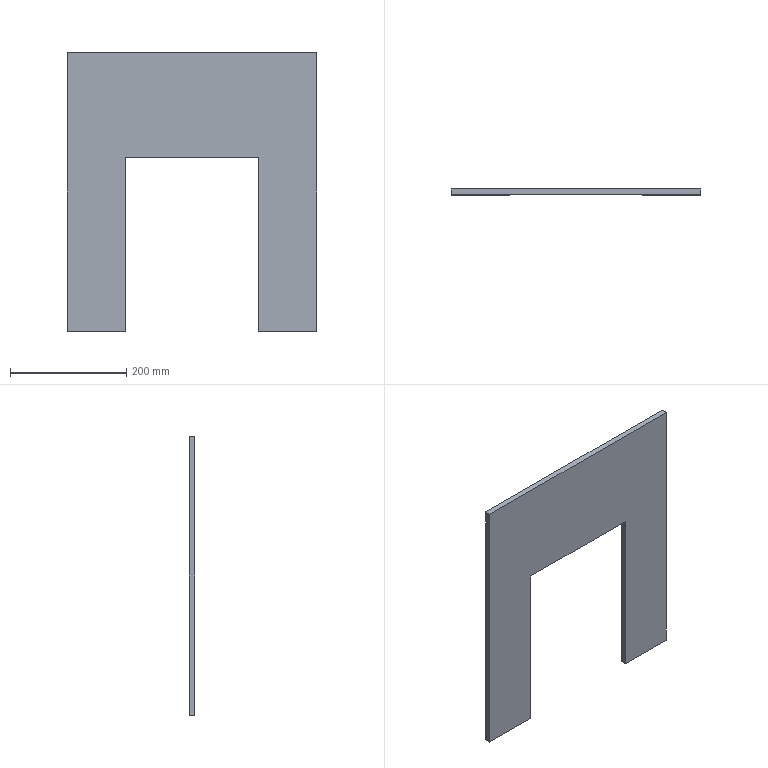Part | STEP file | A14-054 | 1 solid | 10 faces | box 430 x 10 x 480 mm | volume 1374000 mm3 | plane 10
STEP:
#1=CARTESIAN_POINT('',(0.,0.,0.));
#2=DIRECTION('',(0.,0.,1.));
#3=DIRECTION('',(1.,0.,0.));
#4=AXIS2_PLACEMENT_3D('',#1,#2,#3);
#5=CARTESIAN_POINT('',(-115.,-5.,-480.));
#6=VERTEX_POINT('',#5);
#7=CARTESIAN_POINT('',(-215.,-5.,-480.));
#8=VERTEX_POINT('',#7);
#9=CARTESIAN_POINT('',(-215.,-5.,-480.));
#10=DIRECTION('',(-1.,0.,0.));
#11=VECTOR('',#10,1.);
#12=LINE('',#9,#11);
#13=CARTESIAN_POINT('',(-215.,5.,-480.));
#14=DIRECTION('',(0.,0.,1.));
#15=DIRECTION('',(1.,0.,0.));
#16=AXIS2_PLACEMENT_3D('',#13,#14,#15);
#17=PLANE('',#16);
#18=CARTESIAN_POINT('',(0.,-10.));
#19=DIRECTION('',(-1.,0.));
#20=VECTOR('',#19,1.);
#21=LINE('',#18,#20);
#22=(GEOMETRIC_REPRESENTATION_CONTEXT(2)PARAMETRIC_REPRESENTATION_CONTEXT()REPRESENTATION_CONTEXT('',''));
#23=DEFINITIONAL_REPRESENTATION('',(#21),#22);
#24=PCURVE('',#17,#23);
#25=CARTESIAN_POINT('',(0.,-5.,0.));
#26=DIRECTION('',(0.,-1.,0.));
#27=DIRECTION('',(0.,0.,-1.));
#28=AXIS2_PLACEMENT_3D('',#25,#26,#27);
#29=PLANE('',#28);
#30=CARTESIAN_POINT('',(480.,-215.));
#31=DIRECTION('',(0.,-1.));
#32=VECTOR('',#31,1.);
#33=LINE('',#30,#32);
#34=(GEOMETRIC_REPRESENTATION_CONTEXT(2)PARAMETRIC_REPRESENTATION_CONTEXT()REPRESENTATION_CONTEXT('',''));
#35=DEFINITIONAL_REPRESENTATION('',(#33),#34);
#36=PCURVE('',#29,#35);
#37=SURFACE_CURVE('',#12,(#24,#36),.PCURVE_S1.);
#38=EDGE_CURVE('',#6,#8,#37,.T.);
#39=ORIENTED_EDGE('',*,*,#38,.T.);
#40=CARTESIAN_POINT('',(-215.,5.,-480.));
#41=VERTEX_POINT('',#40);
#42=CARTESIAN_POINT('',(-215.,5.,-480.));
#43=DIRECTION('',(0.,-1.,0.));
#44=VECTOR('',#43,1.);
#45=LINE('',#42,#44);
#46=CARTESIAN_POINT('',(0.,0.));
#47=DIRECTION('',(0.,-1.));
#48=VECTOR('',#47,1.);
#49=LINE('',#46,#48);
#50=(GEOMETRIC_REPRESENTATION_CONTEXT(2)PARAMETRIC_REPRESENTATION_CONTEXT()REPRESENTATION_CONTEXT('',''));
#51=DEFINITIONAL_REPRESENTATION('',(#49),#50);
#52=PCURVE('',#17,#51);
#53=CARTESIAN_POINT('',(-215.,5.,0.));
#54=DIRECTION('',(1.,0.,0.));
#55=DIRECTION('',(0.,0.,-1.));
#56=AXIS2_PLACEMENT_3D('',#53,#54,#55);
#57=PLANE('',#56);
#58=CARTESIAN_POINT('',(480.,0.));
#59=DIRECTION('',(0.,-1.));
#60=VECTOR('',#59,1.);
#61=LINE('',#58,#60);
#62=(GEOMETRIC_REPRESENTATION_CONTEXT(2)PARAMETRIC_REPRESENTATION_CONTEXT()REPRESENTATION_CONTEXT('',''));
#63=DEFINITIONAL_REPRESENTATION('',(#61),#62);
#64=PCURVE('',#57,#63);
#65=SURFACE_CURVE('',#45,(#52,#64),.PCURVE_S1.);
#66=EDGE_CURVE('',#41,#8,#65,.T.);
#67=ORIENTED_EDGE('',*,*,#66,.F.);
#68=CARTESIAN_POINT('',(-115.,5.,-480.));
#69=VERTEX_POINT('',#68);
#70=CARTESIAN_POINT('',(-215.,5.,-480.));
#71=DIRECTION('',(-1.,0.,0.));
#72=VECTOR('',#71,1.);
#73=LINE('',#70,#72);
#74=CARTESIAN_POINT('',(0.,0.));
#75=DIRECTION('',(-1.,0.));
#76=VECTOR('',#75,1.);
#77=LINE('',#74,#76);
#78=(GEOMETRIC_REPRESENTATION_CONTEXT(2)PARAMETRIC_REPRESENTATION_CONTEXT()REPRESENTATION_CONTEXT('',''));
#79=DEFINITIONAL_REPRESENTATION('',(#77),#78);
#80=PCURVE('',#17,#79);
#81=CARTESIAN_POINT('',(0.,5.,0.));
#82=DIRECTION('',(0.,-1.,0.));
#83=DIRECTION('',(0.,0.,-1.));
#84=AXIS2_PLACEMENT_3D('',#81,#82,#83);
#85=PLANE('',#84);
#86=CARTESIAN_POINT('',(480.,-215.));
#87=DIRECTION('',(0.,-1.));
#88=VECTOR('',#87,1.);
#89=LINE('',#86,#88);
#90=(GEOMETRIC_REPRESENTATION_CONTEXT(2)PARAMETRIC_REPRESENTATION_CONTEXT()REPRESENTATION_CONTEXT('',''));
#91=DEFINITIONAL_REPRESENTATION('',(#89),#90);
#92=PCURVE('',#85,#91);
#93=SURFACE_CURVE('',#73,(#80,#92),.PCURVE_S1.);
#94=EDGE_CURVE('',#69,#41,#93,.T.);
#95=ORIENTED_EDGE('',*,*,#94,.F.);
#96=CARTESIAN_POINT('',(-115.,5.,-480.));
#97=DIRECTION('',(0.,-1.,0.));
#98=VECTOR('',#97,1.);
#99=LINE('',#96,#98);
#100=CARTESIAN_POINT('',(100.,0.));
#101=DIRECTION('',(0.,-1.));
#102=VECTOR('',#101,1.);
#103=LINE('',#100,#102);
#104=(GEOMETRIC_REPRESENTATION_CONTEXT(2)PARAMETRIC_REPRESENTATION_CONTEXT()REPRESENTATION_CONTEXT('',''));
#105=DEFINITIONAL_REPRESENTATION('',(#103),#104);
#106=PCURVE('',#17,#105);
#107=CARTESIAN_POINT('',(-115.,5.,-480.));
#108=DIRECTION('',(-1.,0.,0.));
#109=DIRECTION('',(0.,0.,1.));
#110=AXIS2_PLACEMENT_3D('',#107,#108,#109);
#111=PLANE('',#110);
#112=CARTESIAN_POINT('',(0.,0.));
#113=DIRECTION('',(0.,-1.));
#114=VECTOR('',#113,1.);
#115=LINE('',#112,#114);
#116=(GEOMETRIC_REPRESENTATION_CONTEXT(2)PARAMETRIC_REPRESENTATION_CONTEXT()REPRESENTATION_CONTEXT('',''));
#117=DEFINITIONAL_REPRESENTATION('',(#115),#116);
#118=PCURVE('',#111,#117);
#119=SURFACE_CURVE('',#99,(#106,#118),.PCURVE_S1.);
#120=EDGE_CURVE('',#69,#6,#119,.T.);
#121=ORIENTED_EDGE('',*,*,#120,.T.);
#122=EDGE_LOOP('',(#39,#67,#95,#121));
#123=FACE_BOUND('',#122,.T.);
#124=ADVANCED_FACE('',(#123),#17,.F.);
#125=CARTESIAN_POINT('',(-215.,-5.,0.));
#126=VERTEX_POINT('',#125);
#127=CARTESIAN_POINT('',(-215.,-5.,0.));
#128=DIRECTION('',(0.,0.,1.));
#129=VECTOR('',#128,1.);
#130=LINE('',#127,#129);
#131=CARTESIAN_POINT('',(0.,-10.));
#132=DIRECTION('',(-1.,0.));
#133=VECTOR('',#132,1.);
#134=LINE('',#131,#133);
#135=(GEOMETRIC_REPRESENTATION_CONTEXT(2)PARAMETRIC_REPRESENTATION_CONTEXT()REPRESENTATION_CONTEXT('',''));
#136=DEFINITIONAL_REPRESENTATION('',(#134),#135);
#137=PCURVE('',#57,#136);
#138=CARTESIAN_POINT('',(0.,-215.));
#139=DIRECTION('',(-1.,0.));
#140=VECTOR('',#139,1.);
#141=LINE('',#138,#140);
#142=(GEOMETRIC_REPRESENTATION_CONTEXT(2)PARAMETRIC_REPRESENTATION_CONTEXT()REPRESENTATION_CONTEXT('',''));
#143=DEFINITIONAL_REPRESENTATION('',(#141),#142);
#144=PCURVE('',#29,#143);
#145=SURFACE_CURVE('',#130,(#137,#144),.PCURVE_S1.);
#146=EDGE_CURVE('',#8,#126,#145,.T.);
#147=ORIENTED_EDGE('',*,*,#146,.T.);
#148=CARTESIAN_POINT('',(-215.,5.,0.));
#149=VERTEX_POINT('',#148);
#150=CARTESIAN_POINT('',(-215.,5.,0.));
#151=DIRECTION('',(0.,-1.,0.));
#152=VECTOR('',#151,1.);
#153=LINE('',#150,#152);
#154=CARTESIAN_POINT('',(0.,0.));
#155=DIRECTION('',(0.,-1.));
#156=VECTOR('',#155,1.);
#157=LINE('',#154,#156);
#158=(GEOMETRIC_REPRESENTATION_CONTEXT(2)PARAMETRIC_REPRESENTATION_CONTEXT()REPRESENTATION_CONTEXT('',''));
#159=DEFINITIONAL_REPRESENTATION('',(#157),#158);
#160=PCURVE('',#57,#159);
#161=CARTESIAN_POINT('',(215.,5.,0.));
#162=DIRECTION('',(0.,0.,-1.));
#163=DIRECTION('',(-1.,0.,0.));
#164=AXIS2_PLACEMENT_3D('',#161,#162,#163);
#165=PLANE('',#164);
#166=CARTESIAN_POINT('',(430.,0.));
#167=DIRECTION('',(0.,-1.));
#168=VECTOR('',#167,1.);
#169=LINE('',#166,#168);
#170=(GEOMETRIC_REPRESENTATION_CONTEXT(2)PARAMETRIC_REPRESENTATION_CONTEXT()REPRESENTATION_CONTEXT('',''));
#171=DEFINITIONAL_REPRESENTATION('',(#169),#170);
#172=PCURVE('',#165,#171);
#173=SURFACE_CURVE('',#153,(#160,#172),.PCURVE_S1.);
#174=EDGE_CURVE('',#149,#126,#173,.T.);
#175=ORIENTED_EDGE('',*,*,#174,.F.);
#176=CARTESIAN_POINT('',(-215.,5.,0.));
#177=DIRECTION('',(0.,0.,1.));
#178=VECTOR('',#177,1.);
#179=LINE('',#176,#178);
#180=CARTESIAN_POINT('',(0.,0.));
#181=DIRECTION('',(-1.,0.));
#182=VECTOR('',#181,1.);
#183=LINE('',#180,#182);
#184=(GEOMETRIC_REPRESENTATION_CONTEXT(2)PARAMETRIC_REPRESENTATION_CONTEXT()REPRESENTATION_CONTEXT('',''));
#185=DEFINITIONAL_REPRESENTATION('',(#183),#184);
#186=PCURVE('',#57,#185);
#187=CARTESIAN_POINT('',(0.,-215.));
#188=DIRECTION('',(-1.,0.));
#189=VECTOR('',#188,1.);
#190=LINE('',#187,#189);
#191=(GEOMETRIC_REPRESENTATION_CONTEXT(2)PARAMETRIC_REPRESENTATION_CONTEXT()REPRESENTATION_CONTEXT('',''));
#192=DEFINITIONAL_REPRESENTATION('',(#190),#191);
#193=PCURVE('',#85,#192);
#194=SURFACE_CURVE('',#179,(#186,#193),.PCURVE_S1.);
#195=EDGE_CURVE('',#41,#149,#194,.T.);
#196=ORIENTED_EDGE('',*,*,#195,.F.);
#197=ORIENTED_EDGE('',*,*,#66,.T.);
#198=EDGE_LOOP('',(#147,#175,#196,#197));
#199=FACE_BOUND('',#198,.T.);
#200=ADVANCED_FACE('',(#199),#57,.F.);
#201=CARTESIAN_POINT('',(215.,-5.,0.));
#202=VERTEX_POINT('',#201);
#203=CARTESIAN_POINT('',(215.,-5.,0.));
#204=DIRECTION('',(1.,0.,0.));
#205=VECTOR('',#204,1.);
#206=LINE('',#203,#205);
#207=CARTESIAN_POINT('',(0.,-10.));
#208=DIRECTION('',(-1.,0.));
#209=VECTOR('',#208,1.);
#210=LINE('',#207,#209);
#211=(GEOMETRIC_REPRESENTATION_CONTEXT(2)PARAMETRIC_REPRESENTATION_CONTEXT()REPRESENTATION_CONTEXT('',''));
#212=DEFINITIONAL_REPRESENTATION('',(#210),#211);
#213=PCURVE('',#165,#212);
#214=CARTESIAN_POINT('',(0.,215.));
#215=DIRECTION('',(0.,1.));
#216=VECTOR('',#215,1.);
#217=LINE('',#214,#216);
#218=(GEOMETRIC_REPRESENTATION_CONTEXT(2)PARAMETRIC_REPRESENTATION_CONTEXT()REPRESENTATION_CONTEXT('',''));
#219=DEFINITIONAL_REPRESENTATION('',(#217),#218);
#220=PCURVE('',#29,#219);
#221=SURFACE_CURVE('',#206,(#213,#220),.PCURVE_S1.);
#222=EDGE_CURVE('',#126,#202,#221,.T.);
#223=ORIENTED_EDGE('',*,*,#222,.T.);
#224=CARTESIAN_POINT('',(215.,5.,0.));
#225=VERTEX_POINT('',#224);
#226=CARTESIAN_POINT('',(215.,5.,0.));
#227=DIRECTION('',(0.,-1.,0.));
#228=VECTOR('',#227,1.);
#229=LINE('',#226,#228);
#230=CARTESIAN_POINT('',(0.,0.));
#231=DIRECTION('',(0.,-1.));
#232=VECTOR('',#231,1.);
#233=LINE('',#230,#232);
#234=(GEOMETRIC_REPRESENTATION_CONTEXT(2)PARAMETRIC_REPRESENTATION_CONTEXT()REPRESENTATION_CONTEXT('',''));
#235=DEFINITIONAL_REPRESENTATION('',(#233),#234);
#236=PCURVE('',#165,#235);
#237=CARTESIAN_POINT('',(215.,5.,-480.));
#238=DIRECTION('',(-1.,0.,0.));
#239=DIRECTION('',(0.,0.,1.));
#240=AXIS2_PLACEMENT_3D('',#237,#238,#239);
#241=PLANE('',#240);
#242=CARTESIAN_POINT('',(480.,0.));
#243=DIRECTION('',(0.,-1.));
#244=VECTOR('',#243,1.);
#245=LINE('',#242,#244);
#246=(GEOMETRIC_REPRESENTATION_CONTEXT(2)PARAMETRIC_REPRESENTATION_CONTEXT()REPRESENTATION_CONTEXT('',''));
#247=DEFINITIONAL_REPRESENTATION('',(#245),#246);
#248=PCURVE('',#241,#247);
#249=SURFACE_CURVE('',#229,(#236,#248),.PCURVE_S1.);
#250=EDGE_CURVE('',#225,#202,#249,.T.);
#251=ORIENTED_EDGE('',*,*,#250,.F.);
#252=CARTESIAN_POINT('',(215.,5.,0.));
#253=DIRECTION('',(1.,0.,0.));
#254=VECTOR('',#253,1.);
#255=LINE('',#252,#254);
#256=CARTESIAN_POINT('',(0.,0.));
#257=DIRECTION('',(-1.,0.));
#258=VECTOR('',#257,1.);
#259=LINE('',#256,#258);
#260=(GEOMETRIC_REPRESENTATION_CONTEXT(2)PARAMETRIC_REPRESENTATION_CONTEXT()REPRESENTATION_CONTEXT('',''));
#261=DEFINITIONAL_REPRESENTATION('',(#259),#260);
#262=PCURVE('',#165,#261);
#263=CARTESIAN_POINT('',(0.,215.));
#264=DIRECTION('',(0.,1.));
#265=VECTOR('',#264,1.);
#266=LINE('',#263,#265);
#267=(GEOMETRIC_REPRESENTATION_CONTEXT(2)PARAMETRIC_REPRESENTATION_CONTEXT()REPRESENTATION_CONTEXT('',''));
#268=DEFINITIONAL_REPRESENTATION('',(#266),#267);
#269=PCURVE('',#85,#268);
#270=SURFACE_CURVE('',#255,(#262,#269),.PCURVE_S1.);
#271=EDGE_CURVE('',#149,#225,#270,.T.);
#272=ORIENTED_EDGE('',*,*,#271,.F.);
#273=ORIENTED_EDGE('',*,*,#174,.T.);
#274=EDGE_LOOP('',(#223,#251,#272,#273));
#275=FACE_BOUND('',#274,.T.);
#276=ADVANCED_FACE('',(#275),#165,.F.);
#277=CARTESIAN_POINT('',(215.,-5.,-480.));
#278=VERTEX_POINT('',#277);
#279=CARTESIAN_POINT('',(215.,-5.,-480.));
#280=DIRECTION('',(0.,0.,-1.));
#281=VECTOR('',#280,1.);
#282=LINE('',#279,#281);
#283=CARTESIAN_POINT('',(0.,-10.));
#284=DIRECTION('',(-1.,0.));
#285=VECTOR('',#284,1.);
#286=LINE('',#283,#285);
#287=(GEOMETRIC_REPRESENTATION_CONTEXT(2)PARAMETRIC_REPRESENTATION_CONTEXT()REPRESENTATION_CONTEXT('',''));
#288=DEFINITIONAL_REPRESENTATION('',(#286),#287);
#289=PCURVE('',#241,#288);
#290=CARTESIAN_POINT('',(480.,215.));
#291=DIRECTION('',(1.,0.));
#292=VECTOR('',#291,1.);
#293=LINE('',#290,#292);
#294=(GEOMETRIC_REPRESENTATION_CONTEXT(2)PARAMETRIC_REPRESENTATION_CONTEXT()REPRESENTATION_CONTEXT('',''));
#295=DEFINITIONAL_REPRESENTATION('',(#293),#294);
#296=PCURVE('',#29,#295);
#297=SURFACE_CURVE('',#282,(#289,#296),.PCURVE_S1.);
#298=EDGE_CURVE('',#202,#278,#297,.T.);
#299=ORIENTED_EDGE('',*,*,#298,.T.);
#300=CARTESIAN_POINT('',(215.,5.,-480.));
#301=VERTEX_POINT('',#300);
#302=CARTESIAN_POINT('',(215.,5.,-480.));
#303=DIRECTION('',(0.,-1.,0.));
#304=VECTOR('',#303,1.);
#305=LINE('',#302,#304);
#306=CARTESIAN_POINT('',(0.,0.));
#307=DIRECTION('',(0.,-1.));
#308=VECTOR('',#307,1.);
#309=LINE('',#306,#308);
#310=(GEOMETRIC_REPRESENTATION_CONTEXT(2)PARAMETRIC_REPRESENTATION_CONTEXT()REPRESENTATION_CONTEXT('',''));
#311=DEFINITIONAL_REPRESENTATION('',(#309),#310);
#312=PCURVE('',#241,#311);
#313=CARTESIAN_POINT('',(115.,5.,-480.));
#314=DIRECTION('',(0.,0.,1.));
#315=DIRECTION('',(1.,0.,0.));
#316=AXIS2_PLACEMENT_3D('',#313,#314,#315);
#317=PLANE('',#316);
#318=CARTESIAN_POINT('',(100.,0.));
#319=DIRECTION('',(0.,-1.));
#320=VECTOR('',#319,1.);
#321=LINE('',#318,#320);
#322=(GEOMETRIC_REPRESENTATION_CONTEXT(2)PARAMETRIC_REPRESENTATION_CONTEXT()REPRESENTATION_CONTEXT('',''));
#323=DEFINITIONAL_REPRESENTATION('',(#321),#322);
#324=PCURVE('',#317,#323);
#325=SURFACE_CURVE('',#305,(#312,#324),.PCURVE_S1.);
#326=EDGE_CURVE('',#301,#278,#325,.T.);
#327=ORIENTED_EDGE('',*,*,#326,.F.);
#328=CARTESIAN_POINT('',(215.,5.,-480.));
#329=DIRECTION('',(0.,0.,-1.));
#330=VECTOR('',#329,1.);
#331=LINE('',#328,#330);
#332=CARTESIAN_POINT('',(0.,0.));
#333=DIRECTION('',(-1.,0.));
#334=VECTOR('',#333,1.);
#335=LINE('',#332,#334);
#336=(GEOMETRIC_REPRESENTATION_CONTEXT(2)PARAMETRIC_REPRESENTATION_CONTEXT()REPRESENTATION_CONTEXT('',''));
#337=DEFINITIONAL_REPRESENTATION('',(#335),#336);
#338=PCURVE('',#241,#337);
#339=CARTESIAN_POINT('',(480.,215.));
#340=DIRECTION('',(1.,0.));
#341=VECTOR('',#340,1.);
#342=LINE('',#339,#341);
#343=(GEOMETRIC_REPRESENTATION_CONTEXT(2)PARAMETRIC_REPRESENTATION_CONTEXT()REPRESENTATION_CONTEXT('',''));
#344=DEFINITIONAL_REPRESENTATION('',(#342),#343);
#345=PCURVE('',#85,#344);
#346=SURFACE_CURVE('',#331,(#338,#345),.PCURVE_S1.);
#347=EDGE_CURVE('',#225,#301,#346,.T.);
#348=ORIENTED_EDGE('',*,*,#347,.F.);
#349=ORIENTED_EDGE('',*,*,#250,.T.);
#350=EDGE_LOOP('',(#299,#327,#348,#349));
#351=FACE_BOUND('',#350,.T.);
#352=ADVANCED_FACE('',(#351),#241,.F.);
#353=CARTESIAN_POINT('',(115.,-5.,-480.));
#354=VERTEX_POINT('',#353);
#355=CARTESIAN_POINT('',(115.,-5.,-480.));
#356=DIRECTION('',(-1.,0.,0.));
#357=VECTOR('',#356,1.);
#358=LINE('',#355,#357);
#359=CARTESIAN_POINT('',(0.,-10.));
#360=DIRECTION('',(-1.,0.));
#361=VECTOR('',#360,1.);
#362=LINE('',#359,#361);
#363=(GEOMETRIC_REPRESENTATION_CONTEXT(2)PARAMETRIC_REPRESENTATION_CONTEXT()REPRESENTATION_CONTEXT('',''));
#364=DEFINITIONAL_REPRESENTATION('',(#362),#363);
#365=PCURVE('',#317,#364);
#366=CARTESIAN_POINT('',(480.,115.));
#367=DIRECTION('',(0.,-1.));
#368=VECTOR('',#367,1.);
#369=LINE('',#366,#368);
#370=(GEOMETRIC_REPRESENTATION_CONTEXT(2)PARAMETRIC_REPRESENTATION_CONTEXT()REPRESENTATION_CONTEXT('',''));
#371=DEFINITIONAL_REPRESENTATION('',(#369),#370);
#372=PCURVE('',#29,#371);
#373=SURFACE_CURVE('',#358,(#365,#372),.PCURVE_S1.);
#374=EDGE_CURVE('',#278,#354,#373,.T.);
#375=ORIENTED_EDGE('',*,*,#374,.T.);
#376=CARTESIAN_POINT('',(115.,5.,-480.));
#377=VERTEX_POINT('',#376);
#378=CARTESIAN_POINT('',(115.,5.,-480.));
#379=DIRECTION('',(0.,-1.,0.));
#380=VECTOR('',#379,1.);
#381=LINE('',#378,#380);
#382=CARTESIAN_POINT('',(0.,0.));
#383=DIRECTION('',(0.,-1.));
#384=VECTOR('',#383,1.);
#385=LINE('',#382,#384);
#386=(GEOMETRIC_REPRESENTATION_CONTEXT(2)PARAMETRIC_REPRESENTATION_CONTEXT()REPRESENTATION_CONTEXT('',''));
#387=DEFINITIONAL_REPRESENTATION('',(#385),#386);
#388=PCURVE('',#317,#387);
#389=CARTESIAN_POINT('',(115.,5.,-180.));
#390=DIRECTION('',(1.,0.,0.));
#391=DIRECTION('',(0.,0.,-1.));
#392=AXIS2_PLACEMENT_3D('',#389,#390,#391);
#393=PLANE('',#392);
#394=CARTESIAN_POINT('',(300.,0.));
#395=DIRECTION('',(0.,-1.));
#396=VECTOR('',#395,1.);
#397=LINE('',#394,#396);
#398=(GEOMETRIC_REPRESENTATION_CONTEXT(2)PARAMETRIC_REPRESENTATION_CONTEXT()REPRESENTATION_CONTEXT('',''));
#399=DEFINITIONAL_REPRESENTATION('',(#397),#398);
#400=PCURVE('',#393,#399);
#401=SURFACE_CURVE('',#381,(#388,#400),.PCURVE_S1.);
#402=EDGE_CURVE('',#377,#354,#401,.T.);
#403=ORIENTED_EDGE('',*,*,#402,.F.);
#404=CARTESIAN_POINT('',(115.,5.,-480.));
#405=DIRECTION('',(-1.,0.,0.));
#406=VECTOR('',#405,1.);
#407=LINE('',#404,#406);
#408=CARTESIAN_POINT('',(0.,0.));
#409=DIRECTION('',(-1.,0.));
#410=VECTOR('',#409,1.);
#411=LINE('',#408,#410);
#412=(GEOMETRIC_REPRESENTATION_CONTEXT(2)PARAMETRIC_REPRESENTATION_CONTEXT()REPRESENTATION_CONTEXT('',''));
#413=DEFINITIONAL_REPRESENTATION('',(#411),#412);
#414=PCURVE('',#317,#413);
#415=CARTESIAN_POINT('',(480.,115.));
#416=DIRECTION('',(0.,-1.));
#417=VECTOR('',#416,1.);
#418=LINE('',#415,#417);
#419=(GEOMETRIC_REPRESENTATION_CONTEXT(2)PARAMETRIC_REPRESENTATION_CONTEXT()REPRESENTATION_CONTEXT('',''));
#420=DEFINITIONAL_REPRESENTATION('',(#418),#419);
#421=PCURVE('',#85,#420);
#422=SURFACE_CURVE('',#407,(#414,#421),.PCURVE_S1.);
#423=EDGE_CURVE('',#301,#377,#422,.T.);
#424=ORIENTED_EDGE('',*,*,#423,.F.);
#425=ORIENTED_EDGE('',*,*,#326,.T.);
#426=EDGE_LOOP('',(#375,#403,#424,#425));
#427=FACE_BOUND('',#426,.T.);
#428=ADVANCED_FACE('',(#427),#317,.F.);
#429=CARTESIAN_POINT('',(115.,-5.,-180.));
#430=VERTEX_POINT('',#429);
#431=CARTESIAN_POINT('',(115.,-5.,-180.));
#432=DIRECTION('',(0.,0.,1.));
#433=VECTOR('',#432,1.);
#434=LINE('',#431,#433);
#435=CARTESIAN_POINT('',(0.,-10.));
#436=DIRECTION('',(-1.,0.));
#437=VECTOR('',#436,1.);
#438=LINE('',#435,#437);
#439=(GEOMETRIC_REPRESENTATION_CONTEXT(2)PARAMETRIC_REPRESENTATION_CONTEXT()REPRESENTATION_CONTEXT('',''));
#440=DEFINITIONAL_REPRESENTATION('',(#438),#439);
#441=PCURVE('',#393,#440);
#442=CARTESIAN_POINT('',(180.,115.));
#443=DIRECTION('',(-1.,0.));
#444=VECTOR('',#443,1.);
#445=LINE('',#442,#444);
#446=(GEOMETRIC_REPRESENTATION_CONTEXT(2)PARAMETRIC_REPRESENTATION_CONTEXT()REPRESENTATION_CONTEXT('',''));
#447=DEFINITIONAL_REPRESENTATION('',(#445),#446);
#448=PCURVE('',#29,#447);
#449=SURFACE_CURVE('',#434,(#441,#448),.PCURVE_S1.);
#450=EDGE_CURVE('',#354,#430,#449,.T.);
#451=ORIENTED_EDGE('',*,*,#450,.T.);
#452=CARTESIAN_POINT('',(115.,5.,-180.));
#453=VERTEX_POINT('',#452);
#454=CARTESIAN_POINT('',(115.,5.,-180.));
#455=DIRECTION('',(0.,-1.,0.));
#456=VECTOR('',#455,1.);
#457=LINE('',#454,#456);
#458=CARTESIAN_POINT('',(0.,0.));
#459=DIRECTION('',(0.,-1.));
#460=VECTOR('',#459,1.);
#461=LINE('',#458,#460);
#462=(GEOMETRIC_REPRESENTATION_CONTEXT(2)PARAMETRIC_REPRESENTATION_CONTEXT()REPRESENTATION_CONTEXT('',''));
#463=DEFINITIONAL_REPRESENTATION('',(#461),#462);
#464=PCURVE('',#393,#463);
#465=CARTESIAN_POINT('',(-115.,5.,-180.));
#466=DIRECTION('',(0.,0.,1.));
#467=DIRECTION('',(1.,0.,0.));
#468=AXIS2_PLACEMENT_3D('',#465,#466,#467);
#469=PLANE('',#468);
#470=CARTESIAN_POINT('',(230.,0.));
#471=DIRECTION('',(0.,-1.));
#472=VECTOR('',#471,1.);
#473=LINE('',#470,#472);
#474=(GEOMETRIC_REPRESENTATION_CONTEXT(2)PARAMETRIC_REPRESENTATION_CONTEXT()REPRESENTATION_CONTEXT('',''));
#475=DEFINITIONAL_REPRESENTATION('',(#473),#474);
#476=PCURVE('',#469,#475);
#477=SURFACE_CURVE('',#457,(#464,#476),.PCURVE_S1.);
#478=EDGE_CURVE('',#453,#430,#477,.T.);
#479=ORIENTED_EDGE('',*,*,#478,.F.);
#480=CARTESIAN_POINT('',(115.,5.,-180.));
#481=DIRECTION('',(0.,0.,1.));
#482=VECTOR('',#481,1.);
#483=LINE('',#480,#482);
#484=CARTESIAN_POINT('',(0.,0.));
#485=DIRECTION('',(-1.,0.));
#486=VECTOR('',#485,1.);
#487=LINE('',#484,#486);
#488=(GEOMETRIC_REPRESENTATION_CONTEXT(2)PARAMETRIC_REPRESENTATION_CONTEXT()REPRESENTATION_CONTEXT('',''));
#489=DEFINITIONAL_REPRESENTATION('',(#487),#488);
#490=PCURVE('',#393,#489);
#491=CARTESIAN_POINT('',(180.,115.));
#492=DIRECTION('',(-1.,0.));
#493=VECTOR('',#492,1.);
#494=LINE('',#491,#493);
#495=(GEOMETRIC_REPRESENTATION_CONTEXT(2)PARAMETRIC_REPRESENTATION_CONTEXT()REPRESENTATION_CONTEXT('',''));
#496=DEFINITIONAL_REPRESENTATION('',(#494),#495);
#497=PCURVE('',#85,#496);
#498=SURFACE_CURVE('',#483,(#490,#497),.PCURVE_S1.);
#499=EDGE_CURVE('',#377,#453,#498,.T.);
#500=ORIENTED_EDGE('',*,*,#499,.F.);
#501=ORIENTED_EDGE('',*,*,#402,.T.);
#502=EDGE_LOOP('',(#451,#479,#500,#501));
#503=FACE_BOUND('',#502,.T.);
#504=ADVANCED_FACE('',(#503),#393,.F.);
#505=CARTESIAN_POINT('',(-115.,-5.,-180.));
#506=VERTEX_POINT('',#505);
#507=CARTESIAN_POINT('',(-115.,-5.,-180.));
#508=DIRECTION('',(-1.,0.,0.));
#509=VECTOR('',#508,1.);
#510=LINE('',#507,#509);
#511=CARTESIAN_POINT('',(0.,-10.));
#512=DIRECTION('',(-1.,0.));
#513=VECTOR('',#512,1.);
#514=LINE('',#511,#513);
#515=(GEOMETRIC_REPRESENTATION_CONTEXT(2)PARAMETRIC_REPRESENTATION_CONTEXT()REPRESENTATION_CONTEXT('',''));
#516=DEFINITIONAL_REPRESENTATION('',(#514),#515);
#517=PCURVE('',#469,#516);
#518=CARTESIAN_POINT('',(180.,-115.));
#519=DIRECTION('',(0.,-1.));
#520=VECTOR('',#519,1.);
#521=LINE('',#518,#520);
#522=(GEOMETRIC_REPRESENTATION_CONTEXT(2)PARAMETRIC_REPRESENTATION_CONTEXT()REPRESENTATION_CONTEXT('',''));
#523=DEFINITIONAL_REPRESENTATION('',(#521),#522);
#524=PCURVE('',#29,#523);
#525=SURFACE_CURVE('',#510,(#517,#524),.PCURVE_S1.);
#526=EDGE_CURVE('',#430,#506,#525,.T.);
#527=ORIENTED_EDGE('',*,*,#526,.T.);
#528=CARTESIAN_POINT('',(-115.,5.,-180.));
#529=VERTEX_POINT('',#528);
#530=CARTESIAN_POINT('',(-115.,5.,-180.));
#531=DIRECTION('',(0.,-1.,0.));
#532=VECTOR('',#531,1.);
#533=LINE('',#530,#532);
#534=CARTESIAN_POINT('',(0.,0.));
#535=DIRECTION('',(0.,-1.));
#536=VECTOR('',#535,1.);
#537=LINE('',#534,#536);
#538=(GEOMETRIC_REPRESENTATION_CONTEXT(2)PARAMETRIC_REPRESENTATION_CONTEXT()REPRESENTATION_CONTEXT('',''));
#539=DEFINITIONAL_REPRESENTATION('',(#537),#538);
#540=PCURVE('',#469,#539);
#541=CARTESIAN_POINT('',(300.,0.));
#542=DIRECTION('',(0.,-1.));
#543=VECTOR('',#542,1.);
#544=LINE('',#541,#543);
#545=(GEOMETRIC_REPRESENTATION_CONTEXT(2)PARAMETRIC_REPRESENTATION_CONTEXT()REPRESENTATION_CONTEXT('',''));
#546=DEFINITIONAL_REPRESENTATION('',(#544),#545);
#547=PCURVE('',#111,#546);
#548=SURFACE_CURVE('',#533,(#540,#547),.PCURVE_S1.);
#549=EDGE_CURVE('',#529,#506,#548,.T.);
#550=ORIENTED_EDGE('',*,*,#549,.F.);
#551=CARTESIAN_POINT('',(-115.,5.,-180.));
#552=DIRECTION('',(-1.,0.,0.));
#553=VECTOR('',#552,1.);
#554=LINE('',#551,#553);
#555=CARTESIAN_POINT('',(0.,0.));
#556=DIRECTION('',(-1.,0.));
#557=VECTOR('',#556,1.);
#558=LINE('',#555,#557);
#559=(GEOMETRIC_REPRESENTATION_CONTEXT(2)PARAMETRIC_REPRESENTATION_CONTEXT()REPRESENTATION_CONTEXT('',''));
#560=DEFINITIONAL_REPRESENTATION('',(#558),#559);
#561=PCURVE('',#469,#560);
#562=CARTESIAN_POINT('',(180.,-115.));
#563=DIRECTION('',(0.,-1.));
#564=VECTOR('',#563,1.);
#565=LINE('',#562,#564);
#566=(GEOMETRIC_REPRESENTATION_CONTEXT(2)PARAMETRIC_REPRESENTATION_CONTEXT()REPRESENTATION_CONTEXT('',''));
#567=DEFINITIONAL_REPRESENTATION('',(#565),#566);
#568=PCURVE('',#85,#567);
#569=SURFACE_CURVE('',#554,(#561,#568),.PCURVE_S1.);
#570=EDGE_CURVE('',#453,#529,#569,.T.);
#571=ORIENTED_EDGE('',*,*,#570,.F.);
#572=ORIENTED_EDGE('',*,*,#478,.T.);
#573=EDGE_LOOP('',(#527,#550,#571,#572));
#574=FACE_BOUND('',#573,.T.);
#575=ADVANCED_FACE('',(#574),#469,.F.);
#576=CARTESIAN_POINT('',(-115.,-5.,-480.));
#577=DIRECTION('',(0.,0.,-1.));
#578=VECTOR('',#577,1.);
#579=LINE('',#576,#578);
#580=CARTESIAN_POINT('',(0.,-10.));
#581=DIRECTION('',(-1.,0.));
#582=VECTOR('',#581,1.);
#583=LINE('',#580,#582);
#584=(GEOMETRIC_REPRESENTATION_CONTEXT(2)PARAMETRIC_REPRESENTATION_CONTEXT()REPRESENTATION_CONTEXT('',''));
#585=DEFINITIONAL_REPRESENTATION('',(#583),#584);
#586=PCURVE('',#111,#585);
#587=CARTESIAN_POINT('',(480.,-115.));
#588=DIRECTION('',(1.,0.));
#589=VECTOR('',#588,1.);
#590=LINE('',#587,#589);
#591=(GEOMETRIC_REPRESENTATION_CONTEXT(2)PARAMETRIC_REPRESENTATION_CONTEXT()REPRESENTATION_CONTEXT('',''));
#592=DEFINITIONAL_REPRESENTATION('',(#590),#591);
#593=PCURVE('',#29,#592);
#594=SURFACE_CURVE('',#579,(#586,#593),.PCURVE_S1.);
#595=EDGE_CURVE('',#506,#6,#594,.T.);
#596=ORIENTED_EDGE('',*,*,#595,.T.);
#597=ORIENTED_EDGE('',*,*,#120,.F.);
#598=CARTESIAN_POINT('',(-115.,5.,-480.));
#599=DIRECTION('',(0.,0.,-1.));
#600=VECTOR('',#599,1.);
#601=LINE('',#598,#600);
#602=CARTESIAN_POINT('',(0.,0.));
#603=DIRECTION('',(-1.,0.));
#604=VECTOR('',#603,1.);
#605=LINE('',#602,#604);
#606=(GEOMETRIC_REPRESENTATION_CONTEXT(2)PARAMETRIC_REPRESENTATION_CONTEXT()REPRESENTATION_CONTEXT('',''));
#607=DEFINITIONAL_REPRESENTATION('',(#605),#606);
#608=PCURVE('',#111,#607);
#609=CARTESIAN_POINT('',(480.,-115.));
#610=DIRECTION('',(1.,0.));
#611=VECTOR('',#610,1.);
#612=LINE('',#609,#611);
#613=(GEOMETRIC_REPRESENTATION_CONTEXT(2)PARAMETRIC_REPRESENTATION_CONTEXT()REPRESENTATION_CONTEXT('',''));
#614=DEFINITIONAL_REPRESENTATION('',(#612),#613);
#615=PCURVE('',#85,#614);
#616=SURFACE_CURVE('',#601,(#608,#615),.PCURVE_S1.);
#617=EDGE_CURVE('',#529,#69,#616,.T.);
#618=ORIENTED_EDGE('',*,*,#617,.F.);
#619=ORIENTED_EDGE('',*,*,#549,.T.);
#620=EDGE_LOOP('',(#596,#597,#618,#619));
#621=FACE_BOUND('',#620,.T.);
#622=ADVANCED_FACE('',(#621),#111,.F.);
#623=ORIENTED_EDGE('',*,*,#94,.T.);
#624=ORIENTED_EDGE('',*,*,#195,.T.);
#625=ORIENTED_EDGE('',*,*,#271,.T.);
#626=ORIENTED_EDGE('',*,*,#347,.T.);
#627=ORIENTED_EDGE('',*,*,#423,.T.);
#628=ORIENTED_EDGE('',*,*,#499,.T.);
#629=ORIENTED_EDGE('',*,*,#570,.T.);
#630=ORIENTED_EDGE('',*,*,#617,.T.);
#631=EDGE_LOOP('',(#623,#624,#625,#626,#627,#628,#629,#630));
#632=FACE_BOUND('',#631,.T.);
#633=ADVANCED_FACE('',(#632),#85,.F.);
#634=ORIENTED_EDGE('',*,*,#38,.F.);
#635=ORIENTED_EDGE('',*,*,#595,.F.);
#636=ORIENTED_EDGE('',*,*,#526,.F.);
#637=ORIENTED_EDGE('',*,*,#450,.F.);
#638=ORIENTED_EDGE('',*,*,#374,.F.);
#639=ORIENTED_EDGE('',*,*,#298,.F.);
#640=ORIENTED_EDGE('',*,*,#222,.F.);
#641=ORIENTED_EDGE('',*,*,#146,.F.);
#642=EDGE_LOOP('',(#634,#635,#636,#637,#638,#639,#640,#641));
#643=FACE_BOUND('',#642,.T.);
#644=ADVANCED_FACE('',(#643),#29,.T.);
#645=CLOSED_SHELL('',(#124,#200,#276,#352,#428,#504,#575,#622,#633,#644));
#646=MANIFOLD_SOLID_BREP('',#645);
#647=(LENGTH_UNIT()NAMED_UNIT(*)SI_UNIT(.MILLI.,.METRE.));
#648=UNCERTAINTY_MEASURE_WITH_UNIT(LENGTH_MEASURE(0.0000001),#647,'','');
#649=(NAMED_UNIT(*)PLANE_ANGLE_UNIT()SI_UNIT($,.RADIAN.));
#650=(NAMED_UNIT(*)SI_UNIT($,.STERADIAN.)SOLID_ANGLE_UNIT());
#651=(GEOMETRIC_REPRESENTATION_CONTEXT(3)GLOBAL_UNCERTAINTY_ASSIGNED_CONTEXT((#648))GLOBAL_UNIT_ASSIGNED_CONTEXT((#647,#649,#650))REPRESENTATION_CONTEXT('',''));
#652=ADVANCED_BREP_SHAPE_REPRESENTATION('',(#4,#646),#651);